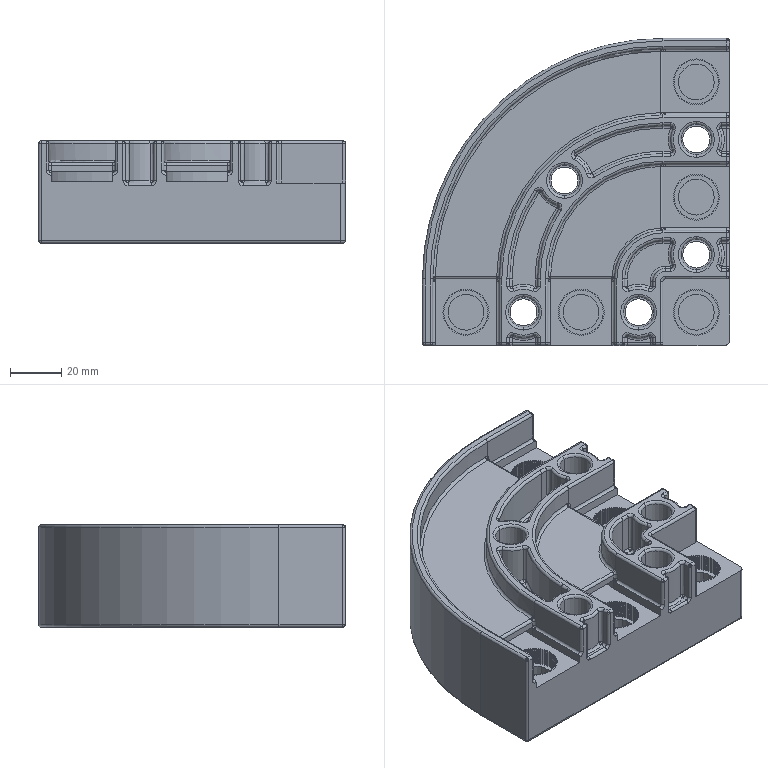Part | SolidWorks | features BaseBody 1 | 1 solid | 2684 faces | box 120 x 120 x 40 mm | volume 221994 mm3 | plane 2017 | cylinder 310 | torus 249 | sphere 100 | spline 8 | commonest cylinder face diameters 2 x162 4 x37 10.5 x20 12 x10 14 x10 15 x10